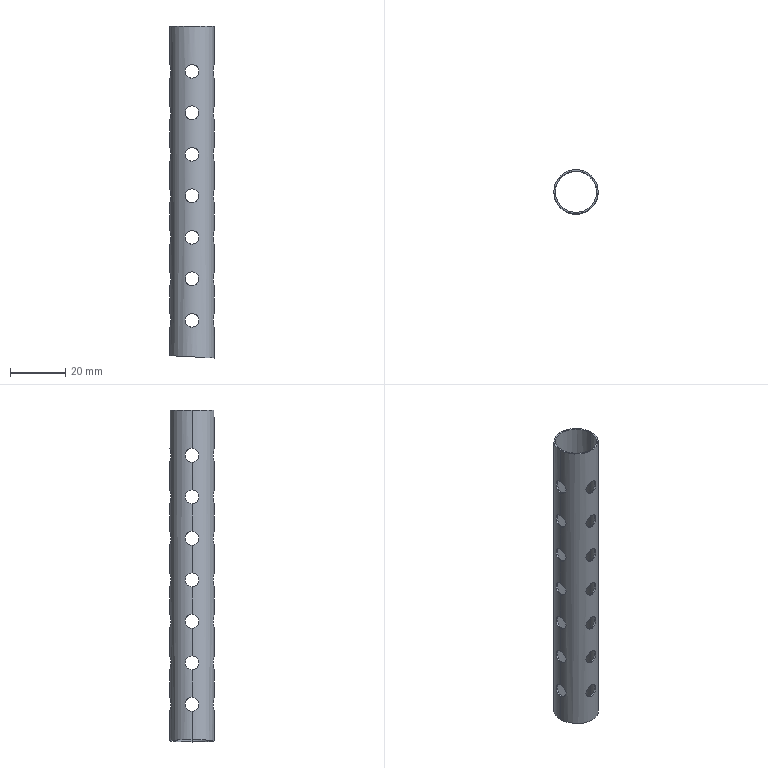Part | SolidWorks | features BaseBody 1 | 1 solid | 62 faces | box 16 x 16 x 120 mm | volume 2633 mm3 | cylinder 60 | plane 2 | commonest cylinder face diameters 5 x56 15 x2 16 x2